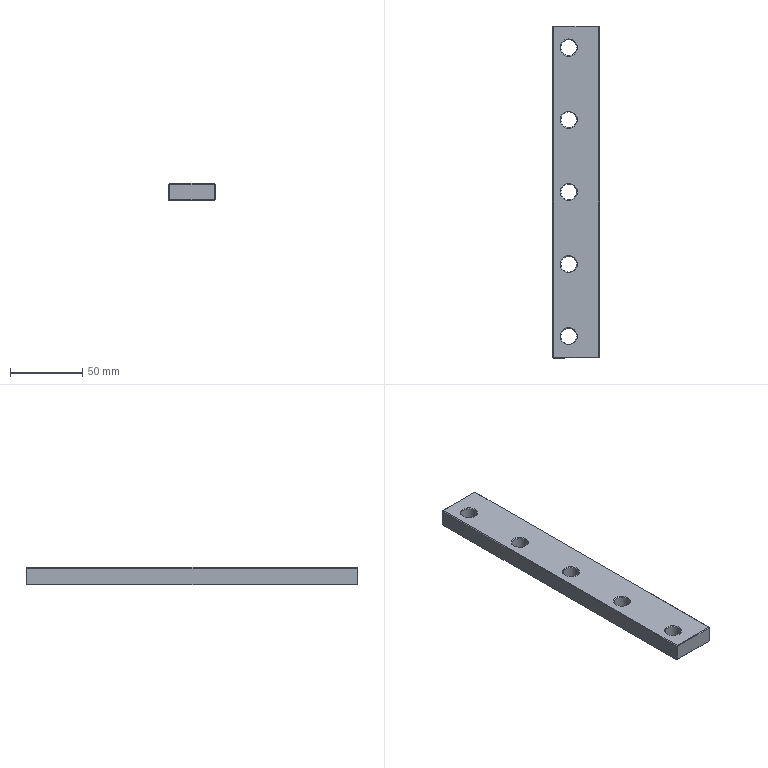Part | SolidWorks | features BaseBody 1 | 1 solid | 53 faces | box 32 x 230 x 12 mm | volume 82466 mm3 | plane 23 | cone 20 | cylinder 10 | commonest cylinder face diameters 11 x10
STEP:
#1=CARTESIAN_POINT('',(79.326,-48.505,0.5));
#2=VERTEX_POINT('',#1);
#3=CARTESIAN_POINT('',(68.326,-48.505,0.5));
#4=VERTEX_POINT('',#3);
#5=CARTESIAN_POINT('',(73.826,-48.505,0.5));
#6=DIRECTION('',(0.,0.,-1.));
#7=DIRECTION('',(-1.,0.,0.));
#8=AXIS2_PLACEMENT_3D('',#5,#6,#7);
#9=CIRCLE('',#8,5.5);
#10=EDGE_CURVE('',#2,#4,#9,.T.);
#11=ORIENTED_EDGE('',*,*,#10,.F.);
#12=CARTESIAN_POINT('',(79.826,-48.505,0.));
#13=VERTEX_POINT('',#12);
#14=CARTESIAN_POINT('',(79.826,-48.505,0.));
#15=DIRECTION('',(0.7071,0.,-0.7071));
#16=VECTOR('',#15,1000.);
#17=LINE('',#14,#16);
#18=EDGE_CURVE('',#2,#13,#17,.T.);
#19=ORIENTED_EDGE('',*,*,#18,.T.);
#20=CARTESIAN_POINT('',(67.826,-48.505,0.));
#21=VERTEX_POINT('',#20);
#22=CARTESIAN_POINT('',(73.826,-48.505,0.));
#23=DIRECTION('',(0.,0.,-1.));
#24=DIRECTION('',(-1.,0.,0.));
#25=AXIS2_PLACEMENT_3D('',#22,#23,#24);
#26=CIRCLE('',#25,6.);
#27=EDGE_CURVE('',#13,#21,#26,.T.);
#28=ORIENTED_EDGE('',*,*,#27,.T.);
#29=CARTESIAN_POINT('',(67.826,-48.505,0.));
#30=DIRECTION('',(-0.7071,0.,-0.7071));
#31=VECTOR('',#30,1000.);
#32=LINE('',#29,#31);
#33=EDGE_CURVE('',#4,#21,#32,.T.);
#34=ORIENTED_EDGE('',*,*,#33,.F.);
#35=EDGE_LOOP('',(#11,#19,#28,#34));
#36=FACE_OUTER_BOUND('',#35,.T.);
#37=CARTESIAN_POINT('',(73.826,-48.505,0.));
#38=DIRECTION('',(0.,0.,-1.));
#39=DIRECTION('',(-1.,0.,0.));
#40=AXIS2_PLACEMENT_3D('',#37,#38,#39);
#41=CONICAL_SURFACE('',#40,6.,0.7854);
#42=ADVANCED_FACE('',(#36),#41,.F.);
#43=CARTESIAN_POINT('',(79.326,1.495,0.5));
#44=VERTEX_POINT('',#43);
#45=CARTESIAN_POINT('',(68.326,1.495,0.5));
#46=VERTEX_POINT('',#45);
#47=CARTESIAN_POINT('',(73.826,1.495,0.5));
#48=DIRECTION('',(0.,0.,-1.));
#49=DIRECTION('',(-1.,0.,0.));
#50=AXIS2_PLACEMENT_3D('',#47,#48,#49);
#51=CIRCLE('',#50,5.5);
#52=EDGE_CURVE('',#44,#46,#51,.T.);
#53=ORIENTED_EDGE('',*,*,#52,.F.);
#54=CARTESIAN_POINT('',(79.826,1.495,0.));
#55=VERTEX_POINT('',#54);
#56=CARTESIAN_POINT('',(79.826,1.495,0.));
#57=DIRECTION('',(0.7071,0.,-0.7071));
#58=VECTOR('',#57,1000.);
#59=LINE('',#56,#58);
#60=EDGE_CURVE('',#44,#55,#59,.T.);
#61=ORIENTED_EDGE('',*,*,#60,.T.);
#62=CARTESIAN_POINT('',(67.826,1.495,0.));
#63=VERTEX_POINT('',#62);
#64=CARTESIAN_POINT('',(73.826,1.495,0.));
#65=DIRECTION('',(0.,0.,-1.));
#66=DIRECTION('',(-1.,0.,0.));
#67=AXIS2_PLACEMENT_3D('',#64,#65,#66);
#68=CIRCLE('',#67,6.);
#69=EDGE_CURVE('',#55,#63,#68,.T.);
#70=ORIENTED_EDGE('',*,*,#69,.T.);
#71=CARTESIAN_POINT('',(67.826,1.495,0.));
#72=DIRECTION('',(-0.7071,0.,-0.7071));
#73=VECTOR('',#72,1000.);
#74=LINE('',#71,#73);
#75=EDGE_CURVE('',#46,#63,#74,.T.);
#76=ORIENTED_EDGE('',*,*,#75,.F.);
#77=EDGE_LOOP('',(#53,#61,#70,#76));
#78=FACE_OUTER_BOUND('',#77,.T.);
#79=CARTESIAN_POINT('',(73.826,1.495,0.));
#80=DIRECTION('',(0.,0.,-1.));
#81=DIRECTION('',(-1.,0.,0.));
#82=AXIS2_PLACEMENT_3D('',#79,#80,#81);
#83=CONICAL_SURFACE('',#82,6.,0.7854);
#84=ADVANCED_FACE('',(#78),#83,.F.);
#85=CARTESIAN_POINT('',(79.326,51.495,0.5));
#86=VERTEX_POINT('',#85);
#87=CARTESIAN_POINT('',(68.326,51.495,0.5));
#88=VERTEX_POINT('',#87);
#89=CARTESIAN_POINT('',(73.826,51.495,0.5));
#90=DIRECTION('',(0.,0.,-1.));
#91=DIRECTION('',(-1.,0.,0.));
#92=AXIS2_PLACEMENT_3D('',#89,#90,#91);
#93=CIRCLE('',#92,5.5);
#94=EDGE_CURVE('',#86,#88,#93,.T.);
#95=ORIENTED_EDGE('',*,*,#94,.F.);
#96=CARTESIAN_POINT('',(79.826,51.495,0.));
#97=VERTEX_POINT('',#96);
#98=CARTESIAN_POINT('',(79.826,51.495,0.));
#99=DIRECTION('',(0.7071,0.,-0.7071));
#100=VECTOR('',#99,1000.);
#101=LINE('',#98,#100);
#102=EDGE_CURVE('',#86,#97,#101,.T.);
#103=ORIENTED_EDGE('',*,*,#102,.T.);
#104=CARTESIAN_POINT('',(67.826,51.495,0.));
#105=VERTEX_POINT('',#104);
#106=CARTESIAN_POINT('',(73.826,51.495,0.));
#107=DIRECTION('',(0.,0.,-1.));
#108=DIRECTION('',(-1.,0.,0.));
#109=AXIS2_PLACEMENT_3D('',#106,#107,#108);
#110=CIRCLE('',#109,6.);
#111=EDGE_CURVE('',#97,#105,#110,.T.);
#112=ORIENTED_EDGE('',*,*,#111,.T.);
#113=CARTESIAN_POINT('',(67.826,51.495,0.));
#114=DIRECTION('',(-0.7071,0.,-0.7071));
#115=VECTOR('',#114,1000.);
#116=LINE('',#113,#115);
#117=EDGE_CURVE('',#88,#105,#116,.T.);
#118=ORIENTED_EDGE('',*,*,#117,.F.);
#119=EDGE_LOOP('',(#95,#103,#112,#118));
#120=FACE_OUTER_BOUND('',#119,.T.);
#121=CARTESIAN_POINT('',(73.826,51.495,0.));
#122=DIRECTION('',(0.,0.,-1.));
#123=DIRECTION('',(-1.,0.,0.));
#124=AXIS2_PLACEMENT_3D('',#121,#122,#123);
#125=CONICAL_SURFACE('',#124,6.,0.7854);
#126=ADVANCED_FACE('',(#120),#125,.F.);
#127=CARTESIAN_POINT('',(79.326,-148.505,0.5));
#128=VERTEX_POINT('',#127);
#129=CARTESIAN_POINT('',(68.326,-148.505,0.5));
#130=VERTEX_POINT('',#129);
#131=CARTESIAN_POINT('',(73.826,-148.505,0.5));
#132=DIRECTION('',(0.,0.,-1.));
#133=DIRECTION('',(-1.,0.,0.));
#134=AXIS2_PLACEMENT_3D('',#131,#132,#133);
#135=CIRCLE('',#134,5.5);
#136=EDGE_CURVE('',#128,#130,#135,.T.);
#137=ORIENTED_EDGE('',*,*,#136,.F.);
#138=CARTESIAN_POINT('',(79.826,-148.505,0.));
#139=VERTEX_POINT('',#138);
#140=CARTESIAN_POINT('',(79.826,-148.505,0.));
#141=DIRECTION('',(0.7071,0.,-0.7071));
#142=VECTOR('',#141,1000.);
#143=LINE('',#140,#142);
#144=EDGE_CURVE('',#128,#139,#143,.T.);
#145=ORIENTED_EDGE('',*,*,#144,.T.);
#146=CARTESIAN_POINT('',(67.826,-148.505,0.));
#147=VERTEX_POINT('',#146);
#148=CARTESIAN_POINT('',(73.826,-148.505,0.));
#149=DIRECTION('',(0.,0.,-1.));
#150=DIRECTION('',(-1.,0.,0.));
#151=AXIS2_PLACEMENT_3D('',#148,#149,#150);
#152=CIRCLE('',#151,6.);
#153=EDGE_CURVE('',#139,#147,#152,.T.);
#154=ORIENTED_EDGE('',*,*,#153,.T.);
#155=CARTESIAN_POINT('',(67.826,-148.505,0.));
#156=DIRECTION('',(-0.7071,0.,-0.7071));
#157=VECTOR('',#156,1000.);
#158=LINE('',#155,#157);
#159=EDGE_CURVE('',#130,#147,#158,.T.);
#160=ORIENTED_EDGE('',*,*,#159,.F.);
#161=EDGE_LOOP('',(#137,#145,#154,#160));
#162=FACE_OUTER_BOUND('',#161,.T.);
#163=CARTESIAN_POINT('',(73.826,-148.505,0.));
#164=DIRECTION('',(0.,0.,-1.));
#165=DIRECTION('',(-1.,0.,0.));
#166=AXIS2_PLACEMENT_3D('',#163,#164,#165);
#167=CONICAL_SURFACE('',#166,6.,0.7854);
#168=ADVANCED_FACE('',(#162),#167,.F.);
#169=CARTESIAN_POINT('',(79.326,-98.505,0.5));
#170=VERTEX_POINT('',#169);
#171=CARTESIAN_POINT('',(68.326,-98.505,0.5));
#172=VERTEX_POINT('',#171);
#173=CARTESIAN_POINT('',(73.826,-98.505,0.5));
#174=DIRECTION('',(0.,0.,-1.));
#175=DIRECTION('',(-1.,0.,0.));
#176=AXIS2_PLACEMENT_3D('',#173,#174,#175);
#177=CIRCLE('',#176,5.5);
#178=EDGE_CURVE('',#170,#172,#177,.T.);
#179=ORIENTED_EDGE('',*,*,#178,.F.);
#180=CARTESIAN_POINT('',(79.826,-98.505,0.));
#181=VERTEX_POINT('',#180);
#182=CARTESIAN_POINT('',(79.826,-98.505,0.));
#183=DIRECTION('',(0.7071,0.,-0.7071));
#184=VECTOR('',#183,1000.);
#185=LINE('',#182,#184);
#186=EDGE_CURVE('',#170,#181,#185,.T.);
#187=ORIENTED_EDGE('',*,*,#186,.T.);
#188=CARTESIAN_POINT('',(67.826,-98.505,0.));
#189=VERTEX_POINT('',#188);
#190=CARTESIAN_POINT('',(73.826,-98.505,0.));
#191=DIRECTION('',(0.,0.,-1.));
#192=DIRECTION('',(-1.,0.,0.));
#193=AXIS2_PLACEMENT_3D('',#190,#191,#192);
#194=CIRCLE('',#193,6.);
#195=EDGE_CURVE('',#181,#189,#194,.T.);
#196=ORIENTED_EDGE('',*,*,#195,.T.);
#197=CARTESIAN_POINT('',(67.826,-98.505,0.));
#198=DIRECTION('',(-0.7071,0.,-0.7071));
#199=VECTOR('',#198,1000.);
#200=LINE('',#197,#199);
#201=EDGE_CURVE('',#172,#189,#200,.T.);
#202=ORIENTED_EDGE('',*,*,#201,.F.);
#203=EDGE_LOOP('',(#179,#187,#196,#202));
#204=FACE_OUTER_BOUND('',#203,.T.);
#205=CARTESIAN_POINT('',(73.826,-98.505,0.));
#206=DIRECTION('',(0.,0.,-1.));
#207=DIRECTION('',(-1.,0.,0.));
#208=AXIS2_PLACEMENT_3D('',#205,#206,#207);
#209=CONICAL_SURFACE('',#208,6.,0.7854);
#210=ADVANCED_FACE('',(#204),#209,.F.);
#211=ORIENTED_EDGE('',*,*,#10,.T.);
#212=CARTESIAN_POINT('',(68.326,-48.505,11.5));
#213=VERTEX_POINT('',#212);
#214=CARTESIAN_POINT('',(68.326,-48.505,0.));
#215=DIRECTION('',(0.,0.,1.));
#216=VECTOR('',#215,1000.);
#217=LINE('',#214,#216);
#218=EDGE_CURVE('',#4,#213,#217,.T.);
#219=ORIENTED_EDGE('',*,*,#218,.T.);
#220=CARTESIAN_POINT('',(73.826,-54.005,11.5));
#221=VERTEX_POINT('',#220);
#222=CARTESIAN_POINT('',(73.826,-48.505,11.5));
#223=DIRECTION('',(0.,0.,-1.));
#224=DIRECTION('',(1.,0.,0.));
#225=AXIS2_PLACEMENT_3D('',#222,#223,#224);
#226=CIRCLE('',#225,5.5);
#227=EDGE_CURVE('',#221,#213,#226,.T.);
#228=ORIENTED_EDGE('',*,*,#227,.F.);
#229=CARTESIAN_POINT('',(79.326,-48.505,11.5));
#230=VERTEX_POINT('',#229);
#231=CARTESIAN_POINT('',(73.826,-48.505,11.5));
#232=DIRECTION('',(0.,0.,-1.));
#233=DIRECTION('',(1.,0.,0.));
#234=AXIS2_PLACEMENT_3D('',#231,#232,#233);
#235=CIRCLE('',#234,5.5);
#236=EDGE_CURVE('',#230,#221,#235,.T.);
#237=ORIENTED_EDGE('',*,*,#236,.F.);
#238=CARTESIAN_POINT('',(79.326,-48.505,0.));
#239=DIRECTION('',(0.,0.,1.));
#240=VECTOR('',#239,1000.);
#241=LINE('',#238,#240);
#242=EDGE_CURVE('',#2,#230,#241,.T.);
#243=ORIENTED_EDGE('',*,*,#242,.F.);
#244=EDGE_LOOP('',(#211,#219,#228,#237,#243));
#245=FACE_OUTER_BOUND('',#244,.T.);
#246=CARTESIAN_POINT('',(73.826,-48.505,0.));
#247=DIRECTION('',(0.,0.,1.));
#248=DIRECTION('',(1.,0.,0.));
#249=AXIS2_PLACEMENT_3D('',#246,#247,#248);
#250=CYLINDRICAL_SURFACE('',#249,5.5);
#251=ADVANCED_FACE('',(#245),#250,.F.);
#252=ORIENTED_EDGE('',*,*,#52,.T.);
#253=CARTESIAN_POINT('',(68.326,1.495,11.5));
#254=VERTEX_POINT('',#253);
#255=CARTESIAN_POINT('',(68.326,1.495,0.));
#256=DIRECTION('',(0.,0.,1.));
#257=VECTOR('',#256,1000.);
#258=LINE('',#255,#257);
#259=EDGE_CURVE('',#46,#254,#258,.T.);
#260=ORIENTED_EDGE('',*,*,#259,.T.);
#261=CARTESIAN_POINT('',(73.826,-4.005,11.5));
#262=VERTEX_POINT('',#261);
#263=CARTESIAN_POINT('',(73.826,1.495,11.5));
#264=DIRECTION('',(0.,0.,-1.));
#265=DIRECTION('',(1.,0.,0.));
#266=AXIS2_PLACEMENT_3D('',#263,#264,#265);
#267=CIRCLE('',#266,5.5);
#268=EDGE_CURVE('',#262,#254,#267,.T.);
#269=ORIENTED_EDGE('',*,*,#268,.F.);
#270=CARTESIAN_POINT('',(79.326,1.495,11.5));
#271=VERTEX_POINT('',#270);
#272=CARTESIAN_POINT('',(73.826,1.495,11.5));
#273=DIRECTION('',(0.,0.,-1.));
#274=DIRECTION('',(1.,0.,0.));
#275=AXIS2_PLACEMENT_3D('',#272,#273,#274);
#276=CIRCLE('',#275,5.5);
#277=EDGE_CURVE('',#271,#262,#276,.T.);
#278=ORIENTED_EDGE('',*,*,#277,.F.);
#279=CARTESIAN_POINT('',(79.326,1.495,0.));
#280=DIRECTION('',(0.,0.,1.));
#281=VECTOR('',#280,1000.);
#282=LINE('',#279,#281);
#283=EDGE_CURVE('',#44,#271,#282,.T.);
#284=ORIENTED_EDGE('',*,*,#283,.F.);
#285=EDGE_LOOP('',(#252,#260,#269,#278,#284));
#286=FACE_OUTER_BOUND('',#285,.T.);
#287=CARTESIAN_POINT('',(73.826,1.495,0.));
#288=DIRECTION('',(0.,0.,1.));
#289=DIRECTION('',(1.,0.,0.));
#290=AXIS2_PLACEMENT_3D('',#287,#288,#289);
#291=CYLINDRICAL_SURFACE('',#290,5.5);
#292=ADVANCED_FACE('',(#286),#291,.F.);
#293=ORIENTED_EDGE('',*,*,#94,.T.);
#294=CARTESIAN_POINT('',(68.326,51.495,11.5));
#295=VERTEX_POINT('',#294);
#296=CARTESIAN_POINT('',(68.326,51.495,0.));
#297=DIRECTION('',(0.,0.,1.));
#298=VECTOR('',#297,1000.);
#299=LINE('',#296,#298);
#300=EDGE_CURVE('',#88,#295,#299,.T.);
#301=ORIENTED_EDGE('',*,*,#300,.T.);
#302=CARTESIAN_POINT('',(73.826,45.995,11.5));
#303=VERTEX_POINT('',#302);
#304=CARTESIAN_POINT('',(73.826,51.495,11.5));
#305=DIRECTION('',(0.,0.,-1.));
#306=DIRECTION('',(1.,0.,0.));
#307=AXIS2_PLACEMENT_3D('',#304,#305,#306);
#308=CIRCLE('',#307,5.5);
#309=EDGE_CURVE('',#303,#295,#308,.T.);
#310=ORIENTED_EDGE('',*,*,#309,.F.);
#311=CARTESIAN_POINT('',(79.326,51.495,11.5));
#312=VERTEX_POINT('',#311);
#313=CARTESIAN_POINT('',(73.826,51.495,11.5));
#314=DIRECTION('',(0.,0.,-1.));
#315=DIRECTION('',(1.,0.,0.));
#316=AXIS2_PLACEMENT_3D('',#313,#314,#315);
#317=CIRCLE('',#316,5.5);
#318=EDGE_CURVE('',#312,#303,#317,.T.);
#319=ORIENTED_EDGE('',*,*,#318,.F.);
#320=CARTESIAN_POINT('',(79.326,51.495,0.));
#321=DIRECTION('',(0.,0.,1.));
#322=VECTOR('',#321,1000.);
#323=LINE('',#320,#322);
#324=EDGE_CURVE('',#86,#312,#323,.T.);
#325=ORIENTED_EDGE('',*,*,#324,.F.);
#326=EDGE_LOOP('',(#293,#301,#310,#319,#325));
#327=FACE_OUTER_BOUND('',#326,.T.);
#328=CARTESIAN_POINT('',(73.826,51.495,0.));
#329=DIRECTION('',(0.,0.,1.));
#330=DIRECTION('',(1.,0.,0.));
#331=AXIS2_PLACEMENT_3D('',#328,#329,#330);
#332=CYLINDRICAL_SURFACE('',#331,5.5);
#333=ADVANCED_FACE('',(#327),#332,.F.);
#334=ORIENTED_EDGE('',*,*,#136,.T.);
#335=CARTESIAN_POINT('',(68.326,-148.505,11.5));
#336=VERTEX_POINT('',#335);
#337=CARTESIAN_POINT('',(68.326,-148.505,0.));
#338=DIRECTION('',(0.,0.,1.));
#339=VECTOR('',#338,1000.);
#340=LINE('',#337,#339);
#341=EDGE_CURVE('',#130,#336,#340,.T.);
#342=ORIENTED_EDGE('',*,*,#341,.T.);
#343=CARTESIAN_POINT('',(73.826,-154.005,11.5));
#344=VERTEX_POINT('',#343);
#345=CARTESIAN_POINT('',(73.826,-148.505,11.5));
#346=DIRECTION('',(0.,0.,-1.));
#347=DIRECTION('',(1.,0.,0.));
#348=AXIS2_PLACEMENT_3D('',#345,#346,#347);
#349=CIRCLE('',#348,5.5);
#350=EDGE_CURVE('',#344,#336,#349,.T.);
#351=ORIENTED_EDGE('',*,*,#350,.F.);
#352=CARTESIAN_POINT('',(79.326,-148.505,11.5));
#353=VERTEX_POINT('',#352);
#354=CARTESIAN_POINT('',(73.826,-148.505,11.5));
#355=DIRECTION('',(0.,0.,-1.));
#356=DIRECTION('',(1.,0.,0.));
#357=AXIS2_PLACEMENT_3D('',#354,#355,#356);
#358=CIRCLE('',#357,5.5);
#359=EDGE_CURVE('',#353,#344,#358,.T.);
#360=ORIENTED_EDGE('',*,*,#359,.F.);
#361=CARTESIAN_POINT('',(79.326,-148.505,0.));
#362=DIRECTION('',(0.,0.,1.));
#363=VECTOR('',#362,1000.);
#364=LINE('',#361,#363);
#365=EDGE_CURVE('',#128,#353,#364,.T.);
#366=ORIENTED_EDGE('',*,*,#365,.F.);
#367=EDGE_LOOP('',(#334,#342,#351,#360,#366));
#368=FACE_OUTER_BOUND('',#367,.T.);
#369=CARTESIAN_POINT('',(73.826,-148.505,0.));
#370=DIRECTION('',(0.,0.,1.));
#371=DIRECTION('',(1.,0.,0.));
#372=AXIS2_PLACEMENT_3D('',#369,#370,#371);
#373=CYLINDRICAL_SURFACE('',#372,5.5);
#374=ADVANCED_FACE('',(#368),#373,.F.);
#375=ORIENTED_EDGE('',*,*,#178,.T.);
#376=CARTESIAN_POINT('',(68.326,-98.505,11.5));
#377=VERTEX_POINT('',#376);
#378=CARTESIAN_POINT('',(68.326,-98.505,0.));
#379=DIRECTION('',(0.,0.,1.));
#380=VECTOR('',#379,1000.);
#381=LINE('',#378,#380);
#382=EDGE_CURVE('',#172,#377,#381,.T.);
#383=ORIENTED_EDGE('',*,*,#382,.T.);
#384=CARTESIAN_POINT('',(73.826,-104.005,11.5));
#385=VERTEX_POINT('',#384);
#386=CARTESIAN_POINT('',(73.826,-98.505,11.5));
#387=DIRECTION('',(0.,0.,-1.));
#388=DIRECTION('',(1.,0.,0.));
#389=AXIS2_PLACEMENT_3D('',#386,#387,#388);
#390=CIRCLE('',#389,5.5);
#391=EDGE_CURVE('',#385,#377,#390,.T.);
#392=ORIENTED_EDGE('',*,*,#391,.F.);
#393=CARTESIAN_POINT('',(79.326,-98.505,11.5));
#394=VERTEX_POINT('',#393);
#395=CARTESIAN_POINT('',(73.826,-98.505,11.5));
#396=DIRECTION('',(0.,0.,-1.));
#397=DIRECTION('',(1.,0.,0.));
#398=AXIS2_PLACEMENT_3D('',#395,#396,#397);
#399=CIRCLE('',#398,5.5);
#400=EDGE_CURVE('',#394,#385,#399,.T.);
#401=ORIENTED_EDGE('',*,*,#400,.F.);
#402=CARTESIAN_POINT('',(79.326,-98.505,0.));
#403=DIRECTION('',(0.,0.,1.));
#404=VECTOR('',#403,1000.);
#405=LINE('',#402,#404);
#406=EDGE_CURVE('',#170,#394,#405,.T.);
#407=ORIENTED_EDGE('',*,*,#406,.F.);
#408=EDGE_LOOP('',(#375,#383,#392,#401,#407));
#409=FACE_OUTER_BOUND('',#408,.T.);
#410=CARTESIAN_POINT('',(73.826,-98.505,0.));
#411=DIRECTION('',(0.,0.,1.));
#412=DIRECTION('',(1.,0.,0.));
#413=AXIS2_PLACEMENT_3D('',#410,#411,#412);
#414=CYLINDRICAL_SURFACE('',#413,5.5);
#415=ADVANCED_FACE('',(#409),#414,.F.);
#416=ORIENTED_EDGE('',*,*,#227,.T.);
#417=CARTESIAN_POINT('',(73.826,-43.005,11.5));
#418=VERTEX_POINT('',#417);
#419=CARTESIAN_POINT('',(73.826,-48.505,11.5));
#420=DIRECTION('',(0.,0.,-1.));
#421=DIRECTION('',(1.,0.,0.));
#422=AXIS2_PLACEMENT_3D('',#419,#420,#421);
#423=CIRCLE('',#422,5.5);
#424=EDGE_CURVE('',#213,#418,#423,.T.);
#425=ORIENTED_EDGE('',*,*,#424,.T.);
#426=CARTESIAN_POINT('',(73.826,-42.505,12.));
#427=VERTEX_POINT('',#426);
#428=CARTESIAN_POINT('',(73.826,-42.505,12.));
#429=DIRECTION('',(0.,0.7071,0.7071));
#430=VECTOR('',#429,1000.);
#431=LINE('',#428,#430);
#432=EDGE_CURVE('',#418,#427,#431,.T.);
#433=ORIENTED_EDGE('',*,*,#432,.T.);
#434=CARTESIAN_POINT('',(73.826,-54.505,12.));
#435=VERTEX_POINT('',#434);
#436=CARTESIAN_POINT('',(73.826,-48.505,12.));
#437=DIRECTION('',(0.,0.,-1.));
#438=DIRECTION('',(0.,-1.,0.));
#439=AXIS2_PLACEMENT_3D('',#436,#437,#438);
#440=CIRCLE('',#439,6.);
#441=EDGE_CURVE('',#435,#427,#440,.T.);
#442=ORIENTED_EDGE('',*,*,#441,.F.);
#443=CARTESIAN_POINT('',(73.826,-54.505,12.));
#444=DIRECTION('',(0.,-0.7071,0.7071));
#445=VECTOR('',#444,1000.);
#446=LINE('',#443,#445);
#447=EDGE_CURVE('',#221,#435,#446,.T.);
#448=ORIENTED_EDGE('',*,*,#447,.F.);
#449=EDGE_LOOP('',(#416,#425,#433,#442,#448));
#450=FACE_OUTER_BOUND('',#449,.T.);
#451=CARTESIAN_POINT('',(73.826,-48.505,12.));
#452=DIRECTION('',(0.,0.,1.));
#453=DIRECTION('',(0.,-1.,0.));
#454=AXIS2_PLACEMENT_3D('',#451,#452,#453);
#455=CONICAL_SURFACE('',#454,6.,0.7854);
#456=ADVANCED_FACE('',(#450),#455,.F.);
#457=ORIENTED_EDGE('',*,*,#268,.T.);
#458=CARTESIAN_POINT('',(73.826,6.995,11.5));
#459=VERTEX_POINT('',#458);
#460=CARTESIAN_POINT('',(73.826,1.495,11.5));
#461=DIRECTION('',(0.,0.,-1.));
#462=DIRECTION('',(1.,0.,0.));
#463=AXIS2_PLACEMENT_3D('',#460,#461,#462);
#464=CIRCLE('',#463,5.5);
#465=EDGE_CURVE('',#254,#459,#464,.T.);
#466=ORIENTED_EDGE('',*,*,#465,.T.);
#467=CARTESIAN_POINT('',(73.826,7.495,12.));
#468=VERTEX_POINT('',#467);
#469=CARTESIAN_POINT('',(73.826,7.495,12.));
#470=DIRECTION('',(0.,0.7071,0.7071));
#471=VECTOR('',#470,1000.);
#472=LINE('',#469,#471);
#473=EDGE_CURVE('',#459,#468,#472,.T.);
#474=ORIENTED_EDGE('',*,*,#473,.T.);
#475=CARTESIAN_POINT('',(73.826,-4.505,12.));
#476=VERTEX_POINT('',#475);
#477=CARTESIAN_POINT('',(73.826,1.495,12.));
#478=DIRECTION('',(0.,0.,-1.));
#479=DIRECTION('',(0.,-1.,0.));
#480=AXIS2_PLACEMENT_3D('',#477,#478,#479);
#481=CIRCLE('',#480,6.);
#482=EDGE_CURVE('',#476,#468,#481,.T.);
#483=ORIENTED_EDGE('',*,*,#482,.F.);
#484=CARTESIAN_POINT('',(73.826,-4.505,12.));
#485=DIRECTION('',(0.,-0.7071,0.7071));
#486=VECTOR('',#485,1000.);
#487=LINE('',#484,#486);
#488=EDGE_CURVE('',#262,#476,#487,.T.);
#489=ORIENTED_EDGE('',*,*,#488,.F.);
#490=EDGE_LOOP('',(#457,#466,#474,#483,#489));
#491=FACE_OUTER_BOUND('',#490,.T.);
#492=CARTESIAN_POINT('',(73.826,1.495,12.));
#493=DIRECTION('',(0.,0.,1.));
#494=DIRECTION('',(0.,-1.,0.));
#495=AXIS2_PLACEMENT_3D('',#492,#493,#494);
#496=CONICAL_SURFACE('',#495,6.,0.7854);
#497=ADVANCED_FACE('',(#491),#496,.F.);
#498=ORIENTED_EDGE('',*,*,#309,.T.);
#499=CARTESIAN_POINT('',(73.826,56.995,11.5));
#500=VERTEX_POINT('',#499);
#501=CARTESIAN_POINT('',(73.826,51.495,11.5));
#502=DIRECTION('',(0.,0.,-1.));
#503=DIRECTION('',(1.,0.,0.));
#504=AXIS2_PLACEMENT_3D('',#501,#502,#503);
#505=CIRCLE('',#504,5.5);
#506=EDGE_CURVE('',#295,#500,#505,.T.);
#507=ORIENTED_EDGE('',*,*,#506,.T.);
#508=CARTESIAN_POINT('',(73.826,57.495,12.));
#509=VERTEX_POINT('',#508);
#510=CARTESIAN_POINT('',(73.826,57.495,12.));
#511=DIRECTION('',(0.,0.7071,0.7071));
#512=VECTOR('',#511,1000.);
#513=LINE('',#510,#512);
#514=EDGE_CURVE('',#500,#509,#513,.T.);
#515=ORIENTED_EDGE('',*,*,#514,.T.);
#516=CARTESIAN_POINT('',(73.826,45.495,12.));
#517=VERTEX_POINT('',#516);
#518=CARTESIAN_POINT('',(73.826,51.495,12.));
#519=DIRECTION('',(0.,0.,-1.));
#520=DIRECTION('',(0.,-1.,0.));
#521=AXIS2_PLACEMENT_3D('',#518,#519,#520);
#522=CIRCLE('',#521,6.);
#523=EDGE_CURVE('',#517,#509,#522,.T.);
#524=ORIENTED_EDGE('',*,*,#523,.F.);
#525=CARTESIAN_POINT('',(73.826,45.495,12.));
#526=DIRECTION('',(0.,-0.7071,0.7071));
#527=VECTOR('',#526,1000.);
#528=LINE('',#525,#527);
#529=EDGE_CURVE('',#303,#517,#528,.T.);
#530=ORIENTED_EDGE('',*,*,#529,.F.);
#531=EDGE_LOOP('',(#498,#507,#515,#524,#530));
#532=FACE_OUTER_BOUND('',#531,.T.);
#533=CARTESIAN_POINT('',(73.826,51.495,12.));
#534=DIRECTION('',(0.,0.,1.));
#535=DIRECTION('',(0.,-1.,0.));
#536=AXIS2_PLACEMENT_3D('',#533,#534,#535);
#537=CONICAL_SURFACE('',#536,6.,0.7854);
#538=ADVANCED_FACE('',(#532),#537,.F.);
#539=ORIENTED_EDGE('',*,*,#350,.T.);
#540=CARTESIAN_POINT('',(73.826,-143.005,11.5));
#541=VERTEX_POINT('',#540);
#542=CARTESIAN_POINT('',(73.826,-148.505,11.5));
#543=DIRECTION('',(0.,0.,-1.));
#544=DIRECTION('',(1.,0.,0.));
#545=AXIS2_PLACEMENT_3D('',#542,#543,#544);
#546=CIRCLE('',#545,5.5);
#547=EDGE_CURVE('',#336,#541,#546,.T.);
#548=ORIENTED_EDGE('',*,*,#547,.T.);
#549=CARTESIAN_POINT('',(73.826,-142.505,12.));
#550=VERTEX_POINT('',#549);
#551=CARTESIAN_POINT('',(73.826,-142.505,12.));
#552=DIRECTION('',(0.,0.7071,0.7071));
#553=VECTOR('',#552,1000.);
#554=LINE('',#551,#553);
#555=EDGE_CURVE('',#541,#550,#554,.T.);
#556=ORIENTED_EDGE('',*,*,#555,.T.);
#557=CARTESIAN_POINT('',(73.826,-154.505,12.));
#558=VERTEX_POINT('',#557);
#559=CARTESIAN_POINT('',(73.826,-148.505,12.));
#560=DIRECTION('',(0.,0.,-1.));
#561=DIRECTION('',(0.,-1.,0.));
#562=AXIS2_PLACEMENT_3D('',#559,#560,#561);
#563=CIRCLE('',#562,6.);
#564=EDGE_CURVE('',#558,#550,#563,.T.);
#565=ORIENTED_EDGE('',*,*,#564,.F.);
#566=CARTESIAN_POINT('',(73.826,-154.505,12.));
#567=DIRECTION('',(0.,-0.7071,0.7071));
#568=VECTOR('',#567,1000.);
#569=LINE('',#566,#568);
#570=EDGE_CURVE('',#344,#558,#569,.T.);
#571=ORIENTED_EDGE('',*,*,#570,.F.);
#572=EDGE_LOOP('',(#539,#548,#556,#565,#571));
#573=FACE_OUTER_BOUND('',#572,.T.);
#574=CARTESIAN_POINT('',(73.826,-148.505,12.));
#575=DIRECTION('',(0.,0.,1.));
#576=DIRECTION('',(0.,-1.,0.));
#577=AXIS2_PLACEMENT_3D('',#574,#575,#576);
#578=CONICAL_SURFACE('',#577,6.,0.7854);
#579=ADVANCED_FACE('',(#573),#578,.F.);
#580=ORIENTED_EDGE('',*,*,#391,.T.);
#581=CARTESIAN_POINT('',(73.826,-93.005,11.5));
#582=VERTEX_POINT('',#581);
#583=CARTESIAN_POINT('',(73.826,-98.505,11.5));
#584=DIRECTION('',(0.,0.,-1.));
#585=DIRECTION('',(1.,0.,0.));
#586=AXIS2_PLACEMENT_3D('',#583,#584,#585);
#587=CIRCLE('',#586,5.5);
#588=EDGE_CURVE('',#377,#582,#587,.T.);
#589=ORIENTED_EDGE('',*,*,#588,.T.);
#590=CARTESIAN_POINT('',(73.826,-92.505,12.));
#591=VERTEX_POINT('',#590);
#592=CARTESIAN_POINT('',(73.826,-92.505,12.));
#593=DIRECTION('',(0.,0.7071,0.7071));
#594=VECTOR('',#593,1000.);
#595=LINE('',#592,#594);
#596=EDGE_CURVE('',#582,#591,#595,.T.);
#597=ORIENTED_EDGE('',*,*,#596,.T.);
#598=CARTESIAN_POINT('',(73.826,-104.505,12.));
#599=VERTEX_POINT('',#598);
#600=CARTESIAN_POINT('',(73.826,-98.505,12.));
#601=DIRECTION('',(0.,0.,-1.));
#602=DIRECTION('',(0.,-1.,0.));
#603=AXIS2_PLACEMENT_3D('',#600,#601,#602);
#604=CIRCLE('',#603,6.);
#605=EDGE_CURVE('',#599,#591,#604,.T.);
#606=ORIENTED_EDGE('',*,*,#605,.F.);
#607=CARTESIAN_POINT('',(73.826,-104.505,12.));
#608=DIRECTION('',(0.,-0.7071,0.7071));
#609=VECTOR('',#608,1000.);
#610=LINE('',#607,#609);
#611=EDGE_CURVE('',#385,#599,#610,.T.);
#612=ORIENTED_EDGE('',*,*,#611,.F.);
#613=EDGE_LOOP('',(#580,#589,#597,#606,#612));
#614=FACE_OUTER_BOUND('',#613,.T.);
#615=CARTESIAN_POINT('',(73.826,-98.505,12.));
#616=DIRECTION('',(0.,0.,1.));
#617=DIRECTION('',(0.,-1.,0.));
#618=AXIS2_PLACEMENT_3D('',#615,#616,#617);
#619=CONICAL_SURFACE('',#618,6.,0.7854);
#620=ADVANCED_FACE('',(#614),#619,.F.);
#621=CARTESIAN_POINT('',(73.826,-48.505,0.));
#622=DIRECTION('',(0.,0.,-1.));
#623=DIRECTION('',(-1.,0.,0.));
#624=AXIS2_PLACEMENT_3D('',#621,#622,#623);
#625=CIRCLE('',#624,6.);
#626=EDGE_CURVE('',#21,#13,#625,.T.);
#627=ORIENTED_EDGE('',*,*,#626,.F.);
#628=ORIENTED_EDGE('',*,*,#27,.F.);
#629=EDGE_LOOP('',(#627,#628));
#630=FACE_BOUND('',#629,.T.);
#631=CARTESIAN_POINT('',(73.826,1.495,0.));
#632=DIRECTION('',(0.,0.,-1.));
#633=DIRECTION('',(-1.,0.,0.));
#634=AXIS2_PLACEMENT_3D('',#631,#632,#633);
#635=CIRCLE('',#634,6.);
#636=EDGE_CURVE('',#63,#55,#635,.T.);
#637=ORIENTED_EDGE('',*,*,#636,.F.);
#638=ORIENTED_EDGE('',*,*,#69,.F.);
#639=EDGE_LOOP('',(#637,#638));
#640=FACE_BOUND('',#639,.T.);
#641=CARTESIAN_POINT('',(73.826,51.495,0.));
#642=DIRECTION('',(0.,0.,-1.));
#643=DIRECTION('',(-1.,0.,0.));
#644=AXIS2_PLACEMENT_3D('',#641,#642,#643);
#645=CIRCLE('',#644,6.);
#646=EDGE_CURVE('',#105,#97,#645,.T.);
#647=ORIENTED_EDGE('',*,*,#646,.F.);
#648=ORIENTED_EDGE('',*,*,#111,.F.);
#649=EDGE_LOOP('',(#647,#648));
#650=FACE_BOUND('',#649,.T.);
#651=CARTESIAN_POINT('',(73.826,-148.505,0.));
#652=DIRECTION('',(0.,0.,-1.));
#653=DIRECTION('',(-1.,0.,0.));
#654=AXIS2_PLACEMENT_3D('',#651,#652,#653);
#655=CIRCLE('',#654,6.);
#656=EDGE_CURVE('',#147,#139,#655,.T.);
#657=ORIENTED_EDGE('',*,*,#656,.F.);
#658=ORIENTED_EDGE('',*,*,#153,.F.);
#659=EDGE_LOOP('',(#657,#658));
#660=FACE_BOUND('',#659,.T.);
#661=CARTESIAN_POINT('',(73.826,-98.505,0.));
#662=DIRECTION('',(0.,0.,-1.));
#663=DIRECTION('',(-1.,0.,0.));
#664=AXIS2_PLACEMENT_3D('',#661,#662,#663);
#665=CIRCLE('',#664,6.);
#666=EDGE_CURVE('',#189,#181,#665,.T.);
#667=ORIENTED_EDGE('',*,*,#666,.F.);
#668=ORIENTED_EDGE('',*,*,#195,.F.);
#669=EDGE_LOOP('',(#667,#668));
#670=FACE_BOUND('',#669,.T.);
#671=CARTESIAN_POINT('',(94.326,-163.005,0.));
#672=VERTEX_POINT('',#671);
#673=CARTESIAN_POINT('',(94.326,65.995,0.));
#674=VERTEX_POINT('',#673);
#675=CARTESIAN_POINT('',(94.326,-48.505,0.));
#676=DIRECTION('',(0.,1.,0.));
#677=VECTOR('',#676,1000.);
#678=LINE('',#675,#677);
#679=EDGE_CURVE('',#672,#674,#678,.T.);
#680=ORIENTED_EDGE('',*,*,#679,.F.);
#681=CARTESIAN_POINT('',(62.826,-163.005,0.));
#682=VERTEX_POINT('',#681);
#683=CARTESIAN_POINT('',(78.826,-163.005,0.));
#684=DIRECTION('',(1.,0.,0.));
#685=VECTOR('',#684,1000.);
#686=LINE('',#683,#685);
#687=EDGE_CURVE('',#682,#672,#686,.T.);
#688=ORIENTED_EDGE('',*,*,#687,.F.);
#689=CARTESIAN_POINT('',(62.826,65.995,0.));
#690=VERTEX_POINT('',#689);
#691=CARTESIAN_POINT('',(62.826,-48.505,0.));
#692=DIRECTION('',(0.,-1.,0.));
#693=VECTOR('',#692,1000.);
#694=LINE('',#691,#693);
#695=EDGE_CURVE('',#690,#682,#694,.T.);
#696=ORIENTED_EDGE('',*,*,#695,.F.);
#697=CARTESIAN_POINT('',(78.826,65.995,0.));
#698=DIRECTION('',(-1.,0.,0.));
#699=VECTOR('',#698,1000.);
#700=LINE('',#697,#699);
#701=EDGE_CURVE('',#674,#690,#700,.T.);
#702=ORIENTED_EDGE('',*,*,#701,.F.);
#703=EDGE_LOOP('',(#680,#688,#696,#702));
#704=FACE_OUTER_BOUND('',#703,.T.);
#705=CARTESIAN_POINT('',(78.826,-48.505,0.));
#706=DIRECTION('',(0.,0.,1.));
#707=DIRECTION('',(1.,0.,0.));
#708=AXIS2_PLACEMENT_3D('',#705,#706,#707);
#709=PLANE('',#708);
#710=ADVANCED_FACE('',(#630,#640,#650,#660,#670,#704),#709,.F.);
#711=ORIENTED_EDGE('',*,*,#18,.F.);
#712=CARTESIAN_POINT('',(73.826,-48.505,0.5));
#713=DIRECTION('',(0.,0.,-1.));
#714=DIRECTION('',(-1.,0.,0.));
#715=AXIS2_PLACEMENT_3D('',#712,#713,#714);
#716=CIRCLE('',#715,5.5);
#717=EDGE_CURVE('',#4,#2,#716,.T.);
#718=ORIENTED_EDGE('',*,*,#717,.F.);
#719=ORIENTED_EDGE('',*,*,#33,.T.);
#720=ORIENTED_EDGE('',*,*,#626,.T.);
#721=EDGE_LOOP('',(#711,#718,#719,#720));
#722=FACE_OUTER_BOUND('',#721,.T.);
#723=CARTESIAN_POINT('',(73.826,-48.505,0.));
#724=DIRECTION('',(0.,0.,-1.));
#725=DIRECTION('',(-1.,0.,0.));
#726=AXIS2_PLACEMENT_3D('',#723,#724,#725);
#727=CONICAL_SURFACE('',#726,6.,0.7854);
#728=ADVANCED_FACE('',(#722),#727,.F.);
#729=ORIENTED_EDGE('',*,*,#60,.F.);
#730=CARTESIAN_POINT('',(73.826,1.495,0.5));
#731=DIRECTION('',(0.,0.,-1.));
#732=DIRECTION('',(-1.,0.,0.));
#733=AXIS2_PLACEMENT_3D('',#730,#731,#732);
#734=CIRCLE('',#733,5.5);
#735=EDGE_CURVE('',#46,#44,#734,.T.);
#736=ORIENTED_EDGE('',*,*,#735,.F.);
#737=ORIENTED_EDGE('',*,*,#75,.T.);
#738=ORIENTED_EDGE('',*,*,#636,.T.);
#739=EDGE_LOOP('',(#729,#736,#737,#738));
#740=FACE_OUTER_BOUND('',#739,.T.);
#741=CARTESIAN_POINT('',(73.826,1.495,0.));
#742=DIRECTION('',(0.,0.,-1.));
#743=DIRECTION('',(-1.,0.,0.));
#744=AXIS2_PLACEMENT_3D('',#741,#742,#743);
#745=CONICAL_SURFACE('',#744,6.,0.7854);
#746=ADVANCED_FACE('',(#740),#745,.F.);
#747=ORIENTED_EDGE('',*,*,#102,.F.);
#748=CARTESIAN_POINT('',(73.826,51.495,0.5));
#749=DIRECTION('',(0.,0.,-1.));
#750=DIRECTION('',(-1.,0.,0.));
#751=AXIS2_PLACEMENT_3D('',#748,#749,#750);
#752=CIRCLE('',#751,5.5);
#753=EDGE_CURVE('',#88,#86,#752,.T.);
#754=ORIENTED_EDGE('',*,*,#753,.F.);
#755=ORIENTED_EDGE('',*,*,#117,.T.);
#756=ORIENTED_EDGE('',*,*,#646,.T.);
#757=EDGE_LOOP('',(#747,#754,#755,#756));
#758=FACE_OUTER_BOUND('',#757,.T.);
#759=CARTESIAN_POINT('',(73.826,51.495,0.));
#760=DIRECTION('',(0.,0.,-1.));
#761=DIRECTION('',(-1.,0.,0.));
#762=AXIS2_PLACEMENT_3D('',#759,#760,#761);
#763=CONICAL_SURFACE('',#762,6.,0.7854);
#764=ADVANCED_FACE('',(#758),#763,.F.);
#765=ORIENTED_EDGE('',*,*,#144,.F.);
#766=CARTESIAN_POINT('',(73.826,-148.505,0.5));
#767=DIRECTION('',(0.,0.,-1.));
#768=DIRECTION('',(-1.,0.,0.));
#769=AXIS2_PLACEMENT_3D('',#766,#767,#768);
#770=CIRCLE('',#769,5.5);
#771=EDGE_CURVE('',#130,#128,#770,.T.);
#772=ORIENTED_EDGE('',*,*,#771,.F.);
#773=ORIENTED_EDGE('',*,*,#159,.T.);
#774=ORIENTED_EDGE('',*,*,#656,.T.);
#775=EDGE_LOOP('',(#765,#772,#773,#774));
#776=FACE_OUTER_BOUND('',#775,.T.);
#777=CARTESIAN_POINT('',(73.826,-148.505,0.));
#778=DIRECTION('',(0.,0.,-1.));
#779=DIRECTION('',(-1.,0.,0.));
#780=AXIS2_PLACEMENT_3D('',#777,#778,#779);
#781=CONICAL_SURFACE('',#780,6.,0.7854);
#782=ADVANCED_FACE('',(#776),#781,.F.);
#783=ORIENTED_EDGE('',*,*,#186,.F.);
#784=CARTESIAN_POINT('',(73.826,-98.505,0.5));
#785=DIRECTION('',(0.,0.,-1.));
#786=DIRECTION('',(-1.,0.,0.));
#787=AXIS2_PLACEMENT_3D('',#784,#785,#786);
#788=CIRCLE('',#787,5.5);
#789=EDGE_CURVE('',#172,#170,#788,.T.);
#790=ORIENTED_EDGE('',*,*,#789,.F.);
#791=ORIENTED_EDGE('',*,*,#201,.T.);
#792=ORIENTED_EDGE('',*,*,#666,.T.);
#793=EDGE_LOOP('',(#783,#790,#791,#792));
#794=FACE_OUTER_BOUND('',#793,.T.);
#795=CARTESIAN_POINT('',(73.826,-98.505,0.));
#796=DIRECTION('',(0.,0.,-1.));
#797=DIRECTION('',(-1.,0.,0.));
#798=AXIS2_PLACEMENT_3D('',#795,#796,#797);
#799=CONICAL_SURFACE('',#798,6.,0.7854);
#800=ADVANCED_FACE('',(#794),#799,.F.);
#801=ORIENTED_EDGE('',*,*,#701,.T.);
#802=CARTESIAN_POINT('',(63.326,66.495,0.5));
#803=VERTEX_POINT('',#802);
#804=CARTESIAN_POINT('',(63.326,66.495,0.5));
#805=DIRECTION('',(-0.5774,-0.5774,-0.5774));
#806=VECTOR('',#805,1000.);
#807=LINE('',#804,#806);
#808=EDGE_CURVE('',#803,#690,#807,.T.);
#809=ORIENTED_EDGE('',*,*,#808,.F.);
#810=CARTESIAN_POINT('',(94.326,66.495,0.5));
#811=VERTEX_POINT('',#810);
#812=CARTESIAN_POINT('',(70.826,66.495,0.5));
#813=DIRECTION('',(1.,0.,0.));
#814=VECTOR('',#813,1000.);
#815=LINE('',#812,#814);
#816=EDGE_CURVE('',#803,#811,#815,.T.);
#817=ORIENTED_EDGE('',*,*,#816,.T.);
#818=CARTESIAN_POINT('',(94.326,66.245,0.25));
#819=DIRECTION('',(0.,-0.7071,-0.7071));
#820=VECTOR('',#819,1000.);
#821=LINE('',#818,#820);
#822=EDGE_CURVE('',#811,#674,#821,.T.);
#823=ORIENTED_EDGE('',*,*,#822,.T.);
#824=EDGE_LOOP('',(#801,#809,#817,#823));
#825=FACE_OUTER_BOUND('',#824,.T.);
#826=CARTESIAN_POINT('',(70.826,66.245,0.25));
#827=DIRECTION('',(0.,0.7071,-0.7071));
#828=DIRECTION('',(0.,0.7071,0.7071));
#829=AXIS2_PLACEMENT_3D('',#826,#827,#828);
#830=PLANE('',#829);
#831=ADVANCED_FACE('',(#825),#830,.T.);
#832=CARTESIAN_POINT('',(94.826,-163.005,0.5));
#833=VERTEX_POINT('',#832);
#834=CARTESIAN_POINT('',(94.576,-163.005,0.25));
#835=DIRECTION('',(-0.7071,0.,-0.7071));
#836=VECTOR('',#835,1000.);
#837=LINE('',#834,#836);
#838=EDGE_CURVE('',#833,#672,#837,.T.);
#839=ORIENTED_EDGE('',*,*,#838,.T.);
#840=ORIENTED_EDGE('',*,*,#679,.T.);
#841=CARTESIAN_POINT('',(94.826,65.995,0.5));
#842=VERTEX_POINT('',#841);
#843=CARTESIAN_POINT('',(94.576,65.995,0.25));
#844=DIRECTION('',(0.7071,0.,0.7071));
#845=VECTOR('',#844,1000.);
#846=LINE('',#843,#845);
#847=EDGE_CURVE('',#674,#842,#846,.T.);
#848=ORIENTED_EDGE('',*,*,#847,.T.);
#849=CARTESIAN_POINT('',(94.826,8.995,0.5));
#850=DIRECTION('',(0.,-1.,0.));
#851=VECTOR('',#850,1000.);
#852=LINE('',#849,#851);
#853=EDGE_CURVE('',#842,#833,#852,.T.);
#854=ORIENTED_EDGE('',*,*,#853,.T.);
#855=EDGE_LOOP('',(#839,#840,#848,#854));
#856=FACE_OUTER_BOUND('',#855,.T.);
#857=CARTESIAN_POINT('',(94.576,8.995,0.25));
#858=DIRECTION('',(0.7071,0.,-0.7071));
#859=DIRECTION('',(-0.7071,0.,-0.7071));
#860=AXIS2_PLACEMENT_3D('',#857,#858,#859);
#861=PLANE('',#860);
#862=ADVANCED_FACE('',(#856),#861,.T.);
#863=CARTESIAN_POINT('',(94.326,-163.505,0.5));
#864=VERTEX_POINT('',#863);
#865=CARTESIAN_POINT('',(63.326,-163.505,0.5));
#866=VERTEX_POINT('',#865);
#867=CARTESIAN_POINT('',(86.826,-163.505,0.5));
#868=DIRECTION('',(-1.,0.,0.));
#869=VECTOR('',#868,1000.);
#870=LINE('',#867,#869);
#871=EDGE_CURVE('',#864,#866,#870,.T.);
#872=ORIENTED_EDGE('',*,*,#871,.T.);
#873=CARTESIAN_POINT('',(62.826,-163.005,0.));
#874=DIRECTION('',(0.5774,-0.5774,0.5774));
#875=VECTOR('',#874,1000.);
#876=LINE('',#873,#875);
#877=EDGE_CURVE('',#682,#866,#876,.T.);
#878=ORIENTED_EDGE('',*,*,#877,.F.);
#879=ORIENTED_EDGE('',*,*,#687,.T.);
#880=CARTESIAN_POINT('',(94.326,-163.255,0.25));
#881=DIRECTION('',(0.,-0.7071,0.7071));
#882=VECTOR('',#881,1000.);
#883=LINE('',#880,#882);
#884=EDGE_CURVE('',#672,#864,#883,.T.);
#885=ORIENTED_EDGE('',*,*,#884,.T.);
#886=EDGE_LOOP('',(#872,#878,#879,#885));
#887=FACE_OUTER_BOUND('',#886,.T.);
#888=CARTESIAN_POINT('',(86.826,-163.255,0.25));
#889=DIRECTION('',(0.,-0.7071,-0.7071));
#890=DIRECTION('',(0.,0.7071,-0.7071));
#891=AXIS2_PLACEMENT_3D('',#888,#889,#890);
#892=PLANE('',#891);
#893=ADVANCED_FACE('',(#887),#892,.T.);
#894=CARTESIAN_POINT('',(62.826,-163.005,11.5));
#895=VERTEX_POINT('',#894);
#896=CARTESIAN_POINT('',(62.826,-163.005,0.));
#897=DIRECTION('',(0.,0.,1.));
#898=VECTOR('',#897,1000.);
#899=LINE('',#896,#898);
#900=EDGE_CURVE('',#682,#895,#899,.T.);
#901=ORIENTED_EDGE('',*,*,#900,.T.);
#902=CARTESIAN_POINT('',(62.826,65.995,11.5));
#903=VERTEX_POINT('',#902);
#904=CARTESIAN_POINT('',(62.826,-163.505,11.5));
#905=DIRECTION('',(0.,1.,0.));
#906=VECTOR('',#905,1000.);
#907=LINE('',#904,#906);
#908=EDGE_CURVE('',#895,#903,#907,.T.);
#909=ORIENTED_EDGE('',*,*,#908,.T.);
#910=CARTESIAN_POINT('',(62.826,65.995,0.));
#911=DIRECTION('',(0.,0.,-1.));
#912=VECTOR('',#911,1000.);
#913=LINE('',#910,#912);
#914=EDGE_CURVE('',#903,#690,#913,.T.);
#915=ORIENTED_EDGE('',*,*,#914,.T.);
#916=ORIENTED_EDGE('',*,*,#695,.T.);
#917=EDGE_LOOP('',(#901,#909,#915,#916));
#918=FACE_OUTER_BOUND('',#917,.T.);
#919=CARTESIAN_POINT('',(62.826,-163.505,0.));
#920=DIRECTION('',(-1.,0.,0.));
#921=DIRECTION('',(0.,0.,1.));
#922=AXIS2_PLACEMENT_3D('',#919,#920,#921);
#923=PLANE('',#922);
#924=ADVANCED_FACE('',(#918),#923,.T.);
#925=ORIENTED_EDGE('',*,*,#218,.F.);
#926=ORIENTED_EDGE('',*,*,#717,.T.);
#927=ORIENTED_EDGE('',*,*,#242,.T.);
#928=CARTESIAN_POINT('',(73.826,-48.505,11.5));
#929=DIRECTION('',(0.,0.,-1.));
#930=DIRECTION('',(1.,0.,0.));
#931=AXIS2_PLACEMENT_3D('',#928,#929,#930);
#932=CIRCLE('',#931,5.5);
#933=EDGE_CURVE('',#418,#230,#932,.T.);
#934=ORIENTED_EDGE('',*,*,#933,.F.);
#935=ORIENTED_EDGE('',*,*,#424,.F.);
#936=EDGE_LOOP('',(#925,#926,#927,#934,#935));
#937=FACE_OUTER_BOUND('',#936,.T.);
#938=CARTESIAN_POINT('',(73.826,-48.505,0.));
#939=DIRECTION('',(0.,0.,1.));
#940=DIRECTION('',(1.,0.,0.));
#941=AXIS2_PLACEMENT_3D('',#938,#939,#940);
#942=CYLINDRICAL_SURFACE('',#941,5.5);
#943=ADVANCED_FACE('',(#937),#942,.F.);
#944=ORIENTED_EDGE('',*,*,#259,.F.);
#945=ORIENTED_EDGE('',*,*,#735,.T.);
#946=ORIENTED_EDGE('',*,*,#283,.T.);
#947=CARTESIAN_POINT('',(73.826,1.495,11.5));
#948=DIRECTION('',(0.,0.,-1.));
#949=DIRECTION('',(1.,0.,0.));
#950=AXIS2_PLACEMENT_3D('',#947,#948,#949);
#951=CIRCLE('',#950,5.5);
#952=EDGE_CURVE('',#459,#271,#951,.T.);
#953=ORIENTED_EDGE('',*,*,#952,.F.);
#954=ORIENTED_EDGE('',*,*,#465,.F.);
#955=EDGE_LOOP('',(#944,#945,#946,#953,#954));
#956=FACE_OUTER_BOUND('',#955,.T.);
#957=CARTESIAN_POINT('',(73.826,1.495,0.));
#958=DIRECTION('',(0.,0.,1.));
#959=DIRECTION('',(1.,0.,0.));
#960=AXIS2_PLACEMENT_3D('',#957,#958,#959);
#961=CYLINDRICAL_SURFACE('',#960,5.5);
#962=ADVANCED_FACE('',(#956),#961,.F.);
#963=ORIENTED_EDGE('',*,*,#300,.F.);
#964=ORIENTED_EDGE('',*,*,#753,.T.);
#965=ORIENTED_EDGE('',*,*,#324,.T.);
#966=CARTESIAN_POINT('',(73.826,51.495,11.5));
#967=DIRECTION('',(0.,0.,-1.));
#968=DIRECTION('',(1.,0.,0.));
#969=AXIS2_PLACEMENT_3D('',#966,#967,#968);
#970=CIRCLE('',#969,5.5);
#971=EDGE_CURVE('',#500,#312,#970,.T.);
#972=ORIENTED_EDGE('',*,*,#971,.F.);
#973=ORIENTED_EDGE('',*,*,#506,.F.);
#974=EDGE_LOOP('',(#963,#964,#965,#972,#973));
#975=FACE_OUTER_BOUND('',#974,.T.);
#976=CARTESIAN_POINT('',(73.826,51.495,0.));
#977=DIRECTION('',(0.,0.,1.));
#978=DIRECTION('',(1.,0.,0.));
#979=AXIS2_PLACEMENT_3D('',#976,#977,#978);
#980=CYLINDRICAL_SURFACE('',#979,5.5);
#981=ADVANCED_FACE('',(#975),#980,.F.);
#982=ORIENTED_EDGE('',*,*,#341,.F.);
#983=ORIENTED_EDGE('',*,*,#771,.T.);
#984=ORIENTED_EDGE('',*,*,#365,.T.);
#985=CARTESIAN_POINT('',(73.826,-148.505,11.5));
#986=DIRECTION('',(0.,0.,-1.));
#987=DIRECTION('',(1.,0.,0.));
#988=AXIS2_PLACEMENT_3D('',#985,#986,#987);
#989=CIRCLE('',#988,5.5);
#990=EDGE_CURVE('',#541,#353,#989,.T.);
#991=ORIENTED_EDGE('',*,*,#990,.F.);
#992=ORIENTED_EDGE('',*,*,#547,.F.);
#993=EDGE_LOOP('',(#982,#983,#984,#991,#992));
#994=FACE_OUTER_BOUND('',#993,.T.);
#995=CARTESIAN_POINT('',(73.826,-148.505,0.));
#996=DIRECTION('',(0.,0.,1.));
#997=DIRECTION('',(1.,0.,0.));
#998=AXIS2_PLACEMENT_3D('',#995,#996,#997);
#999=CYLINDRICAL_SURFACE('',#998,5.5);
#1000=ADVANCED_FACE('',(#994),#999,.F.);
#1001=ORIENTED_EDGE('',*,*,#382,.F.);
#1002=ORIENTED_EDGE('',*,*,#789,.T.);
#1003=ORIENTED_EDGE('',*,*,#406,.T.);
#1004=CARTESIAN_POINT('',(73.826,-98.505,11.5));
#1005=DIRECTION('',(0.,0.,-1.));
#1006=DIRECTION('',(1.,0.,0.));
#1007=AXIS2_PLACEMENT_3D('',#1004,#1005,#1006);
#1008=CIRCLE('',#1007,5.5);
#1009=EDGE_CURVE('',#582,#394,#1008,.T.);
#1010=ORIENTED_EDGE('',*,*,#1009,.F.);
#1011=ORIENTED_EDGE('',*,*,#588,.F.);
#1012=EDGE_LOOP('',(#1001,#1002,#1003,#1010,#1011));
#1013=FACE_OUTER_BOUND('',#1012,.T.);
#1014=CARTESIAN_POINT('',(73.826,-98.505,0.));
#1015=DIRECTION('',(0.,0.,1.));
#1016=DIRECTION('',(1.,0.,0.));
#1017=AXIS2_PLACEMENT_3D('',#1014,#1015,#1016);
#1018=CYLINDRICAL_SURFACE('',#1017,5.5);
#1019=ADVANCED_FACE('',(#1013),#1018,.F.);
#1020=CARTESIAN_POINT('',(94.576,66.245,0.5));
#1021=DIRECTION('',(-0.7071,0.7071,0.));
#1022=VECTOR('',#1021,1000.);
#1023=LINE('',#1020,#1022);
#1024=EDGE_CURVE('',#842,#811,#1023,.T.);
#1025=ORIENTED_EDGE('',*,*,#1024,.F.);
#1026=ORIENTED_EDGE('',*,*,#847,.F.);
#1027=ORIENTED_EDGE('',*,*,#822,.F.);
#1028=EDGE_LOOP('',(#1025,#1026,#1027));
#1029=FACE_OUTER_BOUND('',#1028,.T.);
#1030=CARTESIAN_POINT('',(94.576,65.995,0.25));
#1031=DIRECTION('',(0.5774,0.5774,-0.5774));
#1032=DIRECTION('',(0.,0.7071,0.7071));
#1033=AXIS2_PLACEMENT_3D('',#1030,#1031,#1032);
#1034=PLANE('',#1033);
#1035=ADVANCED_FACE('',(#1029),#1034,.T.);
#1036=CARTESIAN_POINT('',(63.326,66.495,11.5));
#1037=VERTEX_POINT('',#1036);
#1038=CARTESIAN_POINT('',(63.326,66.495,0.));
#1039=DIRECTION('',(0.,0.,1.));
#1040=VECTOR('',#1039,1000.);
#1041=LINE('',#1038,#1040);
#1042=EDGE_CURVE('',#803,#1037,#1041,.T.);
#1043=ORIENTED_EDGE('',*,*,#1042,.T.);
#1044=CARTESIAN_POINT('',(94.326,66.495,11.5));
#1045=VERTEX_POINT('',#1044);
#1046=CARTESIAN_POINT('',(62.826,66.495,11.5));
#1047=DIRECTION('',(1.,0.,0.));
#1048=VECTOR('',#1047,1000.);
#1049=LINE('',#1046,#1048);
#1050=EDGE_CURVE('',#1037,#1045,#1049,.T.);
#1051=ORIENTED_EDGE('',*,*,#1050,.T.);
#1052=CARTESIAN_POINT('',(94.326,66.495,0.));
#1053=DIRECTION('',(0.,0.,-1.));
#1054=VECTOR('',#1053,1000.);
#1055=LINE('',#1052,#1054);
#1056=EDGE_CURVE('',#1045,#811,#1055,.T.);
#1057=ORIENTED_EDGE('',*,*,#1056,.T.);
#1058=ORIENTED_EDGE('',*,*,#816,.F.);
#1059=EDGE_LOOP('',(#1043,#1051,#1057,#1058));
#1060=FACE_OUTER_BOUND('',#1059,.T.);
#1061=CARTESIAN_POINT('',(62.826,66.495,0.));
#1062=DIRECTION('',(0.,1.,0.));
#1063=DIRECTION('',(0.,0.,1.));
#1064=AXIS2_PLACEMENT_3D('',#1061,#1062,#1063);
#1065=PLANE('',#1064);
#1066=ADVANCED_FACE('',(#1060),#1065,.T.);
#1067=CARTESIAN_POINT('',(94.576,-163.255,0.5));
#1068=DIRECTION('',(0.7071,0.7071,0.));
#1069=VECTOR('',#1068,1000.);
#1070=LINE('',#1067,#1069);
#1071=EDGE_CURVE('',#864,#833,#1070,.T.);
#1072=ORIENTED_EDGE('',*,*,#1071,.F.);
#1073=ORIENTED_EDGE('',*,*,#884,.F.);
#1074=ORIENTED_EDGE('',*,*,#838,.F.);
#1075=EDGE_LOOP('',(#1072,#1073,#1074));
#1076=FACE_OUTER_BOUND('',#1075,.T.);
#1077=CARTESIAN_POINT('',(94.576,-163.005,0.25));
#1078=DIRECTION('',(0.5774,-0.5774,-0.5774));
#1079=DIRECTION('',(0.,0.7071,-0.7071));
#1080=AXIS2_PLACEMENT_3D('',#1077,#1078,#1079);
#1081=PLANE('',#1080);
#1082=ADVANCED_FACE('',(#1076),#1081,.T.);
#1083=ORIENTED_EDGE('',*,*,#853,.F.);
#1084=CARTESIAN_POINT('',(94.826,65.995,11.5));
#1085=VERTEX_POINT('',#1084);
#1086=CARTESIAN_POINT('',(94.826,65.995,0.));
#1087=DIRECTION('',(0.,0.,1.));
#1088=VECTOR('',#1087,1000.);
#1089=LINE('',#1086,#1088);
#1090=EDGE_CURVE('',#842,#1085,#1089,.T.);
#1091=ORIENTED_EDGE('',*,*,#1090,.T.);
#1092=CARTESIAN_POINT('',(94.826,-163.005,11.5));
#1093=VERTEX_POINT('',#1092);
#1094=CARTESIAN_POINT('',(94.826,66.495,11.5));
#1095=DIRECTION('',(0.,-1.,0.));
#1096=VECTOR('',#1095,1000.);
#1097=LINE('',#1094,#1096);
#1098=EDGE_CURVE('',#1085,#1093,#1097,.T.);
#1099=ORIENTED_EDGE('',*,*,#1098,.T.);
#1100=CARTESIAN_POINT('',(94.826,-163.005,0.));
#1101=DIRECTION('',(0.,0.,-1.));
#1102=VECTOR('',#1101,1000.);
#1103=LINE('',#1100,#1102);
#1104=EDGE_CURVE('',#1093,#833,#1103,.T.);
#1105=ORIENTED_EDGE('',*,*,#1104,.T.);
#1106=EDGE_LOOP('',(#1083,#1091,#1099,#1105));
#1107=FACE_OUTER_BOUND('',#1106,.T.);
#1108=CARTESIAN_POINT('',(94.826,66.495,0.));
#1109=DIRECTION('',(1.,0.,0.));
#1110=DIRECTION('',(0.,0.,-1.));
#1111=AXIS2_PLACEMENT_3D('',#1108,#1109,#1110);
#1112=PLANE('',#1111);
#1113=ADVANCED_FACE('',(#1107),#1112,.T.);
#1114=CARTESIAN_POINT('',(63.326,-163.505,11.5));
#1115=VERTEX_POINT('',#1114);
#1116=CARTESIAN_POINT('',(63.326,-163.505,0.));
#1117=DIRECTION('',(0.,0.,-1.));
#1118=VECTOR('',#1117,1000.);
#1119=LINE('',#1116,#1118);
#1120=EDGE_CURVE('',#1115,#866,#1119,.T.);
#1121=ORIENTED_EDGE('',*,*,#1120,.T.);
#1122=ORIENTED_EDGE('',*,*,#871,.F.);
#1123=CARTESIAN_POINT('',(94.326,-163.505,11.5));
#1124=VERTEX_POINT('',#1123);
#1125=CARTESIAN_POINT('',(94.326,-163.505,0.));
#1126=DIRECTION('',(0.,0.,1.));
#1127=VECTOR('',#1126,1000.);
#1128=LINE('',#1125,#1127);
#1129=EDGE_CURVE('',#864,#1124,#1128,.T.);
#1130=ORIENTED_EDGE('',*,*,#1129,.T.);
#1131=CARTESIAN_POINT('',(94.826,-163.505,11.5));
#1132=DIRECTION('',(-1.,0.,0.));
#1133=VECTOR('',#1132,1000.);
#1134=LINE('',#1131,#1133);
#1135=EDGE_CURVE('',#1124,#1115,#1134,.T.);
#1136=ORIENTED_EDGE('',*,*,#1135,.T.);
#1137=EDGE_LOOP('',(#1121,#1122,#1130,#1136));
#1138=FACE_OUTER_BOUND('',#1137,.T.);
#1139=CARTESIAN_POINT('',(94.826,-163.505,0.));
#1140=DIRECTION('',(0.,-1.,0.));
#1141=DIRECTION('',(1.,0.,0.));
#1142=AXIS2_PLACEMENT_3D('',#1139,#1140,#1141);
#1143=PLANE('',#1142);
#1144=ADVANCED_FACE('',(#1138),#1143,.T.);
#1145=CARTESIAN_POINT('',(63.326,-163.005,12.));
#1146=VERTEX_POINT('',#1145);
#1147=CARTESIAN_POINT('',(63.076,-163.005,11.75));
#1148=DIRECTION('',(0.7071,0.,0.7071));
#1149=VECTOR('',#1148,1000.);
#1150=LINE('',#1147,#1149);
#1151=EDGE_CURVE('',#895,#1146,#1150,.T.);
#1152=ORIENTED_EDGE('',*,*,#1151,.T.);
#1153=CARTESIAN_POINT('',(63.326,65.995,12.));
#1154=VERTEX_POINT('',#1153);
#1155=CARTESIAN_POINT('',(63.326,-106.005,12.));
#1156=DIRECTION('',(0.,1.,0.));
#1157=VECTOR('',#1156,1000.);
#1158=LINE('',#1155,#1157);
#1159=EDGE_CURVE('',#1146,#1154,#1158,.T.);
#1160=ORIENTED_EDGE('',*,*,#1159,.T.);
#1161=CARTESIAN_POINT('',(63.076,65.995,11.75));
#1162=DIRECTION('',(-0.7071,0.,-0.7071));
#1163=VECTOR('',#1162,1000.);
#1164=LINE('',#1161,#1163);
#1165=EDGE_CURVE('',#1154,#903,#1164,.T.);
#1166=ORIENTED_EDGE('',*,*,#1165,.T.);
#1167=ORIENTED_EDGE('',*,*,#908,.F.);
#1168=EDGE_LOOP('',(#1152,#1160,#1166,#1167));
#1169=FACE_OUTER_BOUND('',#1168,.T.);
#1170=CARTESIAN_POINT('',(63.076,-106.005,11.75));
#1171=DIRECTION('',(-0.7071,0.,0.7071));
#1172=DIRECTION('',(0.7071,0.,0.7071));
#1173=AXIS2_PLACEMENT_3D('',#1170,#1171,#1172);
#1174=PLANE('',#1173);
#1175=ADVANCED_FACE('',(#1169),#1174,.T.);
#1176=ORIENTED_EDGE('',*,*,#900,.F.);
#1177=ORIENTED_EDGE('',*,*,#877,.T.);
#1178=ORIENTED_EDGE('',*,*,#1120,.F.);
#1179=CARTESIAN_POINT('',(63.076,-163.255,11.5));
#1180=DIRECTION('',(-0.7071,0.7071,0.));
#1181=VECTOR('',#1180,1000.);
#1182=LINE('',#1179,#1181);
#1183=EDGE_CURVE('',#1115,#895,#1182,.T.);
#1184=ORIENTED_EDGE('',*,*,#1183,.T.);
#1185=EDGE_LOOP('',(#1176,#1177,#1178,#1184));
#1186=FACE_OUTER_BOUND('',#1185,.T.);
#1187=CARTESIAN_POINT('',(63.076,-163.255,0.));
#1188=DIRECTION('',(-0.7071,-0.7071,0.));
#1189=DIRECTION('',(0.7071,-0.7071,0.));
#1190=AXIS2_PLACEMENT_3D('',#1187,#1188,#1189);
#1191=PLANE('',#1190);
#1192=ADVANCED_FACE('',(#1186),#1191,.T.);
#1193=ORIENTED_EDGE('',*,*,#1042,.F.);
#1194=ORIENTED_EDGE('',*,*,#808,.T.);
#1195=ORIENTED_EDGE('',*,*,#914,.F.);
#1196=CARTESIAN_POINT('',(63.076,66.245,11.5));
#1197=DIRECTION('',(0.7071,0.7071,0.));
#1198=VECTOR('',#1197,1000.);
#1199=LINE('',#1196,#1198);
#1200=EDGE_CURVE('',#903,#1037,#1199,.T.);
#1201=ORIENTED_EDGE('',*,*,#1200,.T.);
#1202=EDGE_LOOP('',(#1193,#1194,#1195,#1201));
#1203=FACE_OUTER_BOUND('',#1202,.T.);
#1204=CARTESIAN_POINT('',(63.076,66.245,0.));
#1205=DIRECTION('',(-0.7071,0.7071,0.));
#1206=DIRECTION('',(-0.7071,-0.7071,0.));
#1207=AXIS2_PLACEMENT_3D('',#1204,#1205,#1206);
#1208=PLANE('',#1207);
#1209=ADVANCED_FACE('',(#1203),#1208,.T.);
#1210=ORIENTED_EDGE('',*,*,#432,.F.);
#1211=ORIENTED_EDGE('',*,*,#933,.T.);
#1212=ORIENTED_EDGE('',*,*,#236,.T.);
#1213=ORIENTED_EDGE('',*,*,#447,.T.);
#1214=CARTESIAN_POINT('',(73.826,-48.505,12.));
#1215=DIRECTION('',(0.,0.,-1.));
#1216=DIRECTION('',(0.,-1.,0.));
#1217=AXIS2_PLACEMENT_3D('',#1214,#1215,#1216);
#1218=CIRCLE('',#1217,6.);
#1219=EDGE_CURVE('',#427,#435,#1218,.T.);
#1220=ORIENTED_EDGE('',*,*,#1219,.F.);
#1221=EDGE_LOOP('',(#1210,#1211,#1212,#1213,#1220));
#1222=FACE_OUTER_BOUND('',#1221,.T.);
#1223=CARTESIAN_POINT('',(73.826,-48.505,12.));
#1224=DIRECTION('',(0.,0.,1.));
#1225=DIRECTION('',(0.,-1.,0.));
#1226=AXIS2_PLACEMENT_3D('',#1223,#1224,#1225);
#1227=CONICAL_SURFACE('',#1226,6.,0.7854);
#1228=ADVANCED_FACE('',(#1222),#1227,.F.);
#1229=ORIENTED_EDGE('',*,*,#473,.F.);
#1230=ORIENTED_EDGE('',*,*,#952,.T.);
#1231=ORIENTED_EDGE('',*,*,#277,.T.);
#1232=ORIENTED_EDGE('',*,*,#488,.T.);
#1233=CARTESIAN_POINT('',(73.826,1.495,12.));
#1234=DIRECTION('',(0.,0.,-1.));
#1235=DIRECTION('',(0.,-1.,0.));
#1236=AXIS2_PLACEMENT_3D('',#1233,#1234,#1235);
#1237=CIRCLE('',#1236,6.);
#1238=EDGE_CURVE('',#468,#476,#1237,.T.);
#1239=ORIENTED_EDGE('',*,*,#1238,.F.);
#1240=EDGE_LOOP('',(#1229,#1230,#1231,#1232,#1239));
#1241=FACE_OUTER_BOUND('',#1240,.T.);
#1242=CARTESIAN_POINT('',(73.826,1.495,12.));
#1243=DIRECTION('',(0.,0.,1.));
#1244=DIRECTION('',(0.,-1.,0.));
#1245=AXIS2_PLACEMENT_3D('',#1242,#1243,#1244);
#1246=CONICAL_SURFACE('',#1245,6.,0.7854);
#1247=ADVANCED_FACE('',(#1241),#1246,.F.);
#1248=ORIENTED_EDGE('',*,*,#514,.F.);
#1249=ORIENTED_EDGE('',*,*,#971,.T.);
#1250=ORIENTED_EDGE('',*,*,#318,.T.);
#1251=ORIENTED_EDGE('',*,*,#529,.T.);
#1252=CARTESIAN_POINT('',(73.826,51.495,12.));
#1253=DIRECTION('',(0.,0.,-1.));
#1254=DIRECTION('',(0.,-1.,0.));
#1255=AXIS2_PLACEMENT_3D('',#1252,#1253,#1254);
#1256=CIRCLE('',#1255,6.);
#1257=EDGE_CURVE('',#509,#517,#1256,.T.);
#1258=ORIENTED_EDGE('',*,*,#1257,.F.);
#1259=EDGE_LOOP('',(#1248,#1249,#1250,#1251,#1258));
#1260=FACE_OUTER_BOUND('',#1259,.T.);
#1261=CARTESIAN_POINT('',(73.826,51.495,12.));
#1262=DIRECTION('',(0.,0.,1.));
#1263=DIRECTION('',(0.,-1.,0.));
#1264=AXIS2_PLACEMENT_3D('',#1261,#1262,#1263);
#1265=CONICAL_SURFACE('',#1264,6.,0.7854);
#1266=ADVANCED_FACE('',(#1260),#1265,.F.);
#1267=ORIENTED_EDGE('',*,*,#555,.F.);
#1268=ORIENTED_EDGE('',*,*,#990,.T.);
#1269=ORIENTED_EDGE('',*,*,#359,.T.);
#1270=ORIENTED_EDGE('',*,*,#570,.T.);
#1271=CARTESIAN_POINT('',(73.826,-148.505,12.));
#1272=DIRECTION('',(0.,0.,-1.));
#1273=DIRECTION('',(0.,-1.,0.));
#1274=AXIS2_PLACEMENT_3D('',#1271,#1272,#1273);
#1275=CIRCLE('',#1274,6.);
#1276=EDGE_CURVE('',#550,#558,#1275,.T.);
#1277=ORIENTED_EDGE('',*,*,#1276,.F.);
#1278=EDGE_LOOP('',(#1267,#1268,#1269,#1270,#1277));
#1279=FACE_OUTER_BOUND('',#1278,.T.);
#1280=CARTESIAN_POINT('',(73.826,-148.505,12.));
#1281=DIRECTION('',(0.,0.,1.));
#1282=DIRECTION('',(0.,-1.,0.));
#1283=AXIS2_PLACEMENT_3D('',#1280,#1281,#1282);
#1284=CONICAL_SURFACE('',#1283,6.,0.7854);
#1285=ADVANCED_FACE('',(#1279),#1284,.F.);
#1286=ORIENTED_EDGE('',*,*,#596,.F.);
#1287=ORIENTED_EDGE('',*,*,#1009,.T.);
#1288=ORIENTED_EDGE('',*,*,#400,.T.);
#1289=ORIENTED_EDGE('',*,*,#611,.T.);
#1290=CARTESIAN_POINT('',(73.826,-98.505,12.));
#1291=DIRECTION('',(0.,0.,-1.));
#1292=DIRECTION('',(0.,-1.,0.));
#1293=AXIS2_PLACEMENT_3D('',#1290,#1291,#1292);
#1294=CIRCLE('',#1293,6.);
#1295=EDGE_CURVE('',#591,#599,#1294,.T.);
#1296=ORIENTED_EDGE('',*,*,#1295,.F.);
#1297=EDGE_LOOP('',(#1286,#1287,#1288,#1289,#1296));
#1298=FACE_OUTER_BOUND('',#1297,.T.);
#1299=CARTESIAN_POINT('',(73.826,-98.505,12.));
#1300=DIRECTION('',(0.,0.,1.));
#1301=DIRECTION('',(0.,-1.,0.));
#1302=AXIS2_PLACEMENT_3D('',#1299,#1300,#1301);
#1303=CONICAL_SURFACE('',#1302,6.,0.7854);
#1304=ADVANCED_FACE('',(#1298),#1303,.F.);
#1305=CARTESIAN_POINT('',(63.326,66.245,11.75));
#1306=DIRECTION('',(0.,-0.7071,0.7071));
#1307=VECTOR('',#1306,1000.);
#1308=LINE('',#1305,#1307);
#1309=EDGE_CURVE('',#1037,#1154,#1308,.T.);
#1310=ORIENTED_EDGE('',*,*,#1309,.T.);
#1311=CARTESIAN_POINT('',(94.326,65.995,12.));
#1312=VERTEX_POINT('',#1311);
#1313=CARTESIAN_POINT('',(70.826,65.995,12.));
#1314=DIRECTION('',(1.,0.,0.));
#1315=VECTOR('',#1314,1000.);
#1316=LINE('',#1313,#1315);
#1317=EDGE_CURVE('',#1154,#1312,#1316,.T.);
#1318=ORIENTED_EDGE('',*,*,#1317,.T.);
#1319=CARTESIAN_POINT('',(94.326,66.245,11.75));
#1320=DIRECTION('',(0.,0.7071,-0.7071));
#1321=VECTOR('',#1320,1000.);
#1322=LINE('',#1319,#1321);
#1323=EDGE_CURVE('',#1312,#1045,#1322,.T.);
#1324=ORIENTED_EDGE('',*,*,#1323,.T.);
#1325=ORIENTED_EDGE('',*,*,#1050,.F.);
#1326=EDGE_LOOP('',(#1310,#1318,#1324,#1325));
#1327=FACE_OUTER_BOUND('',#1326,.T.);
#1328=CARTESIAN_POINT('',(70.826,66.245,11.75));
#1329=DIRECTION('',(0.,0.7071,0.7071));
#1330=DIRECTION('',(0.,-0.7071,0.7071));
#1331=AXIS2_PLACEMENT_3D('',#1328,#1329,#1330);
#1332=PLANE('',#1331);
#1333=ADVANCED_FACE('',(#1327),#1332,.T.);
#1334=ORIENTED_EDGE('',*,*,#1024,.T.);
#1335=ORIENTED_EDGE('',*,*,#1056,.F.);
#1336=CARTESIAN_POINT('',(94.576,66.245,11.5));
#1337=DIRECTION('',(0.7071,-0.7071,0.));
#1338=VECTOR('',#1337,1000.);
#1339=LINE('',#1336,#1338);
#1340=EDGE_CURVE('',#1045,#1085,#1339,.T.);
#1341=ORIENTED_EDGE('',*,*,#1340,.T.);
#1342=ORIENTED_EDGE('',*,*,#1090,.F.);
#1343=EDGE_LOOP('',(#1334,#1335,#1341,#1342));
#1344=FACE_OUTER_BOUND('',#1343,.T.);
#1345=CARTESIAN_POINT('',(94.576,66.245,0.));
#1346=DIRECTION('',(0.7071,0.7071,0.));
#1347=DIRECTION('',(-0.7071,0.7071,0.));
#1348=AXIS2_PLACEMENT_3D('',#1345,#1346,#1347);
#1349=PLANE('',#1348);
#1350=ADVANCED_FACE('',(#1344),#1349,.T.);
#1351=ORIENTED_EDGE('',*,*,#1071,.T.);
#1352=ORIENTED_EDGE('',*,*,#1104,.F.);
#1353=CARTESIAN_POINT('',(94.576,-163.255,11.5));
#1354=DIRECTION('',(-0.7071,-0.7071,0.));
#1355=VECTOR('',#1354,1000.);
#1356=LINE('',#1353,#1355);
#1357=EDGE_CURVE('',#1093,#1124,#1356,.T.);
#1358=ORIENTED_EDGE('',*,*,#1357,.T.);
#1359=ORIENTED_EDGE('',*,*,#1129,.F.);
#1360=EDGE_LOOP('',(#1351,#1352,#1358,#1359));
#1361=FACE_OUTER_BOUND('',#1360,.T.);
#1362=CARTESIAN_POINT('',(94.576,-163.255,0.));
#1363=DIRECTION('',(0.7071,-0.7071,0.));
#1364=DIRECTION('',(0.7071,0.7071,0.));
#1365=AXIS2_PLACEMENT_3D('',#1362,#1363,#1364);
#1366=PLANE('',#1365);
#1367=ADVANCED_FACE('',(#1361),#1366,.T.);
#1368=CARTESIAN_POINT('',(94.576,65.995,11.75));
#1369=DIRECTION('',(-0.7071,0.,0.7071));
#1370=VECTOR('',#1369,1000.);
#1371=LINE('',#1368,#1370);
#1372=EDGE_CURVE('',#1085,#1312,#1371,.T.);
#1373=ORIENTED_EDGE('',*,*,#1372,.T.);
#1374=CARTESIAN_POINT('',(94.326,-163.005,12.));
#1375=VERTEX_POINT('',#1374);
#1376=CARTESIAN_POINT('',(94.326,8.995,12.));
#1377=DIRECTION('',(0.,-1.,0.));
#1378=VECTOR('',#1377,1000.);
#1379=LINE('',#1376,#1378);
#1380=EDGE_CURVE('',#1312,#1375,#1379,.T.);
#1381=ORIENTED_EDGE('',*,*,#1380,.T.);
#1382=CARTESIAN_POINT('',(94.576,-163.005,11.75));
#1383=DIRECTION('',(0.7071,0.,-0.7071));
#1384=VECTOR('',#1383,1000.);
#1385=LINE('',#1382,#1384);
#1386=EDGE_CURVE('',#1375,#1093,#1385,.T.);
#1387=ORIENTED_EDGE('',*,*,#1386,.T.);
#1388=ORIENTED_EDGE('',*,*,#1098,.F.);
#1389=EDGE_LOOP('',(#1373,#1381,#1387,#1388));
#1390=FACE_OUTER_BOUND('',#1389,.T.);
#1391=CARTESIAN_POINT('',(94.576,8.995,11.75));
#1392=DIRECTION('',(0.7071,0.,0.7071));
#1393=DIRECTION('',(0.7071,0.,-0.7071));
#1394=AXIS2_PLACEMENT_3D('',#1391,#1392,#1393);
#1395=PLANE('',#1394);
#1396=ADVANCED_FACE('',(#1390),#1395,.T.);
#1397=CARTESIAN_POINT('',(94.326,-163.255,11.75));
#1398=DIRECTION('',(0.,0.7071,0.7071));
#1399=VECTOR('',#1398,1000.);
#1400=LINE('',#1397,#1399);
#1401=EDGE_CURVE('',#1124,#1375,#1400,.T.);
#1402=ORIENTED_EDGE('',*,*,#1401,.T.);
#1403=CARTESIAN_POINT('',(86.826,-163.005,12.));
#1404=DIRECTION('',(-1.,0.,0.));
#1405=VECTOR('',#1404,1000.);
#1406=LINE('',#1403,#1405);
#1407=EDGE_CURVE('',#1375,#1146,#1406,.T.);
#1408=ORIENTED_EDGE('',*,*,#1407,.T.);
#1409=CARTESIAN_POINT('',(63.326,-163.255,11.75));
#1410=DIRECTION('',(0.,-0.7071,-0.7071));
#1411=VECTOR('',#1410,1000.);
#1412=LINE('',#1409,#1411);
#1413=EDGE_CURVE('',#1146,#1115,#1412,.T.);
#1414=ORIENTED_EDGE('',*,*,#1413,.T.);
#1415=ORIENTED_EDGE('',*,*,#1135,.F.);
#1416=EDGE_LOOP('',(#1402,#1408,#1414,#1415));
#1417=FACE_OUTER_BOUND('',#1416,.T.);
#1418=CARTESIAN_POINT('',(86.826,-163.255,11.75));
#1419=DIRECTION('',(0.,-0.7071,0.7071));
#1420=DIRECTION('',(0.,-0.7071,-0.7071));
#1421=AXIS2_PLACEMENT_3D('',#1418,#1419,#1420);
#1422=PLANE('',#1421);
#1423=ADVANCED_FACE('',(#1417),#1422,.T.);
#1424=ORIENTED_EDGE('',*,*,#441,.T.);
#1425=ORIENTED_EDGE('',*,*,#1219,.T.);
#1426=EDGE_LOOP('',(#1424,#1425));
#1427=FACE_BOUND('',#1426,.T.);
#1428=ORIENTED_EDGE('',*,*,#482,.T.);
#1429=ORIENTED_EDGE('',*,*,#1238,.T.);
#1430=EDGE_LOOP('',(#1428,#1429));
#1431=FACE_BOUND('',#1430,.T.);
#1432=ORIENTED_EDGE('',*,*,#523,.T.);
#1433=ORIENTED_EDGE('',*,*,#1257,.T.);
#1434=EDGE_LOOP('',(#1432,#1433));
#1435=FACE_BOUND('',#1434,.T.);
#1436=ORIENTED_EDGE('',*,*,#564,.T.);
#1437=ORIENTED_EDGE('',*,*,#1276,.T.);
#1438=EDGE_LOOP('',(#1436,#1437));
#1439=FACE_BOUND('',#1438,.T.);
#1440=ORIENTED_EDGE('',*,*,#605,.T.);
#1441=ORIENTED_EDGE('',*,*,#1295,.T.);
#1442=EDGE_LOOP('',(#1440,#1441));
#1443=FACE_BOUND('',#1442,.T.);
#1444=ORIENTED_EDGE('',*,*,#1159,.F.);
#1445=ORIENTED_EDGE('',*,*,#1407,.F.);
#1446=ORIENTED_EDGE('',*,*,#1380,.F.);
#1447=ORIENTED_EDGE('',*,*,#1317,.F.);
#1448=EDGE_LOOP('',(#1444,#1445,#1446,#1447));
#1449=FACE_OUTER_BOUND('',#1448,.T.);
#1450=CARTESIAN_POINT('',(78.826,-48.505,12.));
#1451=DIRECTION('',(0.,0.,1.));
#1452=DIRECTION('',(1.,0.,0.));
#1453=AXIS2_PLACEMENT_3D('',#1450,#1451,#1452);
#1454=PLANE('',#1453);
#1455=ADVANCED_FACE('',(#1427,#1431,#1435,#1439,#1443,#1449),#1454,.T.);
#1456=ORIENTED_EDGE('',*,*,#1413,.F.);
#1457=ORIENTED_EDGE('',*,*,#1151,.F.);
#1458=ORIENTED_EDGE('',*,*,#1183,.F.);
#1459=EDGE_LOOP('',(#1456,#1457,#1458));
#1460=FACE_OUTER_BOUND('',#1459,.T.);
#1461=CARTESIAN_POINT('',(63.076,-163.255,11.5));
#1462=DIRECTION('',(-0.5774,-0.5774,0.5774));
#1463=DIRECTION('',(0.7071,0.,0.7071));
#1464=AXIS2_PLACEMENT_3D('',#1461,#1462,#1463);
#1465=PLANE('',#1464);
#1466=ADVANCED_FACE('',(#1460),#1465,.T.);
#1467=ORIENTED_EDGE('',*,*,#1309,.F.);
#1468=ORIENTED_EDGE('',*,*,#1200,.F.);
#1469=ORIENTED_EDGE('',*,*,#1165,.F.);
#1470=EDGE_LOOP('',(#1467,#1468,#1469));
#1471=FACE_OUTER_BOUND('',#1470,.T.);
#1472=CARTESIAN_POINT('',(63.076,66.245,11.5));
#1473=DIRECTION('',(-0.5774,0.5774,0.5774));
#1474=DIRECTION('',(0.,-0.7071,0.7071));
#1475=AXIS2_PLACEMENT_3D('',#1472,#1473,#1474);
#1476=PLANE('',#1475);
#1477=ADVANCED_FACE('',(#1471),#1476,.T.);
#1478=ORIENTED_EDGE('',*,*,#1372,.F.);
#1479=ORIENTED_EDGE('',*,*,#1340,.F.);
#1480=ORIENTED_EDGE('',*,*,#1323,.F.);
#1481=EDGE_LOOP('',(#1478,#1479,#1480));
#1482=FACE_OUTER_BOUND('',#1481,.T.);
#1483=CARTESIAN_POINT('',(94.576,66.245,11.5));
#1484=DIRECTION('',(0.5774,0.5774,0.5774));
#1485=DIRECTION('',(-0.7071,0.7071,0.));
#1486=AXIS2_PLACEMENT_3D('',#1483,#1484,#1485);
#1487=PLANE('',#1486);
#1488=ADVANCED_FACE('',(#1482),#1487,.T.);
#1489=ORIENTED_EDGE('',*,*,#1386,.F.);
#1490=ORIENTED_EDGE('',*,*,#1401,.F.);
#1491=ORIENTED_EDGE('',*,*,#1357,.F.);
#1492=EDGE_LOOP('',(#1489,#1490,#1491));
#1493=FACE_OUTER_BOUND('',#1492,.T.);
#1494=CARTESIAN_POINT('',(94.576,-163.255,11.5));
#1495=DIRECTION('',(0.5774,-0.5774,0.5774));
#1496=DIRECTION('',(0.7071,0.,-0.7071));
#1497=AXIS2_PLACEMENT_3D('',#1494,#1495,#1496);
#1498=PLANE('',#1497);
#1499=ADVANCED_FACE('',(#1493),#1498,.T.);
#1500=CLOSED_SHELL('',(#42,#84,#126,#168,#210,#251,#292,#333,#374,#415,#456,#497,#538,#579,#620,#710,#728,#746,#764,#782,#800,#831,#862,#893,#924,#943,#962,#981,#1000,#1019,#1035,#1066,#1082,#1113,#1144,#1175,#1192,#1209,#1228,#1247,#1266,#1285,#1304,#1333,#1350,#1367,#1396,#1423,#1455,#1466,#1477,#1488,#1499));
#1501=MANIFOLD_SOLID_BREP('',#1500);
#1502=CARTESIAN_POINT('',(0.,0.,0.));
#1503=DIRECTION('',(0.,0.,1.));
#1504=DIRECTION('',(1.,0.,0.));
#1505=AXIS2_PLACEMENT_3D('',#1502,#1503,#1504);
#1506=(LENGTH_UNIT()NAMED_UNIT(*)SI_UNIT(.MILLI.,.METRE.));
#1507=UNCERTAINTY_MEASURE_WITH_UNIT(LENGTH_MEASURE(0.00001),#1506,'','');
#1508=(NAMED_UNIT(*)PLANE_ANGLE_UNIT()SI_UNIT($,.RADIAN.));
#1509=(NAMED_UNIT(*)SI_UNIT($,.STERADIAN.)SOLID_ANGLE_UNIT());
#1510=(GEOMETRIC_REPRESENTATION_CONTEXT(3)GLOBAL_UNCERTAINTY_ASSIGNED_CONTEXT((#1507))GLOBAL_UNIT_ASSIGNED_CONTEXT((#1506,#1508,#1509))REPRESENTATION_CONTEXT('',''));
#1511=ADVANCED_BREP_SHAPE_REPRESENTATION('',(#1501,#1505),#1510);